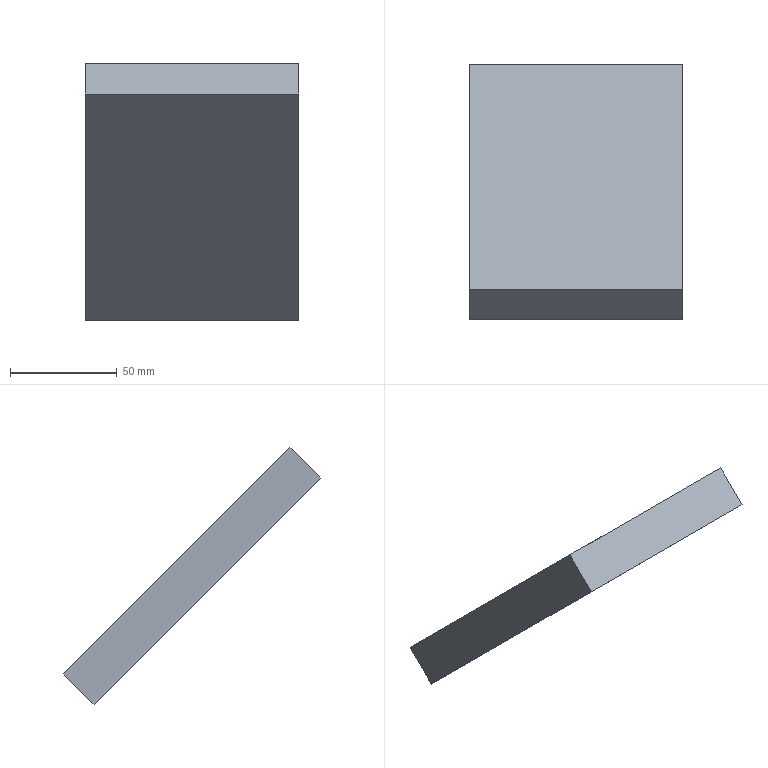Part | NX | features solid 2 | 1 solid | 6 faces | box 100 x 120.208 x 120.208 mm | volume 300000 mm3 | plane 6
STEP:
#1=CARTESIAN_POINT('',(730.,940.563,-169.939));
#2=VERTEX_POINT('',#1);
#3=CARTESIAN_POINT('',(730.,954.706,-155.797));
#4=VERTEX_POINT('',#3);
#5=CARTESIAN_POINT('',(730.,940.563,-169.939));
#6=DIRECTION('',(0.,0.7071,0.7071));
#7=VECTOR('',#6,1000.);
#8=LINE('',#5,#7);
#9=EDGE_CURVE('',#2,#4,#8,.T.);
#10=ORIENTED_EDGE('',*,*,#9,.T.);
#11=CARTESIAN_POINT('',(630.,954.706,-155.797));
#12=VERTEX_POINT('',#11);
#13=CARTESIAN_POINT('',(630.,954.706,-155.797));
#14=DIRECTION('',(1.,0.,0.));
#15=VECTOR('',#14,1000.);
#16=LINE('',#13,#15);
#17=EDGE_CURVE('',#12,#4,#16,.T.);
#18=ORIENTED_EDGE('',*,*,#17,.F.);
#19=CARTESIAN_POINT('',(630.,940.563,-169.939));
#20=VERTEX_POINT('',#19);
#21=CARTESIAN_POINT('',(630.,940.563,-169.939));
#22=DIRECTION('',(0.,0.7071,0.7071));
#23=VECTOR('',#22,1000.);
#24=LINE('',#21,#23);
#25=EDGE_CURVE('',#20,#12,#24,.T.);
#26=ORIENTED_EDGE('',*,*,#25,.F.);
#27=CARTESIAN_POINT('',(630.,940.563,-169.939));
#28=DIRECTION('',(1.,0.,0.));
#29=VECTOR('',#28,1000.);
#30=LINE('',#27,#29);
#31=EDGE_CURVE('',#20,#2,#30,.T.);
#32=ORIENTED_EDGE('',*,*,#31,.T.);
#33=EDGE_LOOP('',(#10,#18,#26,#32));
#34=FACE_BOUND('',#33,.T.);
#35=CARTESIAN_POINT('',(630.,940.563,-169.939));
#36=DIRECTION('',(0.,-0.7071,0.7071));
#37=DIRECTION('',(0.,-0.7071,-0.7071));
#38=AXIS2_PLACEMENT_3D('',#35,#36,#37);
#39=PLANE('',#38);
#40=ADVANCED_FACE('',(#34),#39,.T.);
#41=CARTESIAN_POINT('',(730.,1060.772,-261.863));
#42=VERTEX_POINT('',#41);
#43=CARTESIAN_POINT('',(730.,954.706,-155.797));
#44=DIRECTION('',(0.,0.7071,-0.7071));
#45=VECTOR('',#44,1000.);
#46=LINE('',#43,#45);
#47=EDGE_CURVE('',#4,#42,#46,.T.);
#48=ORIENTED_EDGE('',*,*,#47,.T.);
#49=CARTESIAN_POINT('',(630.,1060.772,-261.863));
#50=VERTEX_POINT('',#49);
#51=CARTESIAN_POINT('',(630.,1060.772,-261.863));
#52=DIRECTION('',(1.,0.,0.));
#53=VECTOR('',#52,1000.);
#54=LINE('',#51,#53);
#55=EDGE_CURVE('',#50,#42,#54,.T.);
#56=ORIENTED_EDGE('',*,*,#55,.F.);
#57=CARTESIAN_POINT('',(630.,954.706,-155.797));
#58=DIRECTION('',(0.,0.7071,-0.7071));
#59=VECTOR('',#58,1000.);
#60=LINE('',#57,#59);
#61=EDGE_CURVE('',#12,#50,#60,.T.);
#62=ORIENTED_EDGE('',*,*,#61,.F.);
#63=ORIENTED_EDGE('',*,*,#17,.T.);
#64=EDGE_LOOP('',(#48,#56,#62,#63));
#65=FACE_BOUND('',#64,.T.);
#66=CARTESIAN_POINT('',(630.,954.706,-155.797));
#67=DIRECTION('',(0.,0.7071,0.7071));
#68=DIRECTION('',(0.,-0.7071,0.7071));
#69=AXIS2_PLACEMENT_3D('',#66,#67,#68);
#70=PLANE('',#69);
#71=ADVANCED_FACE('',(#65),#70,.T.);
#72=CARTESIAN_POINT('',(730.,1046.63,-276.005));
#73=VERTEX_POINT('',#72);
#74=CARTESIAN_POINT('',(730.,1046.63,-276.005));
#75=DIRECTION('',(0.,0.7071,0.7071));
#76=VECTOR('',#75,1000.);
#77=LINE('',#74,#76);
#78=EDGE_CURVE('',#73,#42,#77,.T.);
#79=ORIENTED_EDGE('',*,*,#78,.F.);
#80=CARTESIAN_POINT('',(630.,1046.63,-276.005));
#81=VERTEX_POINT('',#80);
#82=CARTESIAN_POINT('',(630.,1046.63,-276.005));
#83=DIRECTION('',(1.,0.,0.));
#84=VECTOR('',#83,1000.);
#85=LINE('',#82,#84);
#86=EDGE_CURVE('',#81,#73,#85,.T.);
#87=ORIENTED_EDGE('',*,*,#86,.F.);
#88=CARTESIAN_POINT('',(630.,1046.63,-276.005));
#89=DIRECTION('',(0.,0.7071,0.7071));
#90=VECTOR('',#89,1000.);
#91=LINE('',#88,#90);
#92=EDGE_CURVE('',#81,#50,#91,.T.);
#93=ORIENTED_EDGE('',*,*,#92,.T.);
#94=ORIENTED_EDGE('',*,*,#55,.T.);
#95=EDGE_LOOP('',(#79,#87,#93,#94));
#96=FACE_BOUND('',#95,.T.);
#97=CARTESIAN_POINT('',(630.,1046.63,-276.005));
#98=DIRECTION('',(0.,-0.7071,0.7071));
#99=DIRECTION('',(0.,-0.7071,-0.7071));
#100=AXIS2_PLACEMENT_3D('',#97,#98,#99);
#101=PLANE('',#100);
#102=ADVANCED_FACE('',(#96),#101,.F.);
#103=CARTESIAN_POINT('',(730.,940.563,-169.939));
#104=DIRECTION('',(0.,0.7071,-0.7071));
#105=VECTOR('',#104,1000.);
#106=LINE('',#103,#105);
#107=EDGE_CURVE('',#2,#73,#106,.T.);
#108=ORIENTED_EDGE('',*,*,#107,.F.);
#109=ORIENTED_EDGE('',*,*,#31,.F.);
#110=CARTESIAN_POINT('',(630.,940.563,-169.939));
#111=DIRECTION('',(0.,0.7071,-0.7071));
#112=VECTOR('',#111,1000.);
#113=LINE('',#110,#112);
#114=EDGE_CURVE('',#20,#81,#113,.T.);
#115=ORIENTED_EDGE('',*,*,#114,.T.);
#116=ORIENTED_EDGE('',*,*,#86,.T.);
#117=EDGE_LOOP('',(#108,#109,#115,#116));
#118=FACE_BOUND('',#117,.T.);
#119=CARTESIAN_POINT('',(630.,940.563,-169.939));
#120=DIRECTION('',(0.,0.7071,0.7071));
#121=DIRECTION('',(0.,-0.7071,0.7071));
#122=AXIS2_PLACEMENT_3D('',#119,#120,#121);
#123=PLANE('',#122);
#124=ADVANCED_FACE('',(#118),#123,.F.);
#125=ORIENTED_EDGE('',*,*,#25,.T.);
#126=ORIENTED_EDGE('',*,*,#61,.T.);
#127=ORIENTED_EDGE('',*,*,#92,.F.);
#128=ORIENTED_EDGE('',*,*,#114,.F.);
#129=EDGE_LOOP('',(#125,#126,#127,#128));
#130=FACE_BOUND('',#129,.T.);
#131=CARTESIAN_POINT('',(630.,940.563,-169.939));
#132=DIRECTION('',(1.,0.,0.));
#133=DIRECTION('',(0.,0.,1.));
#134=AXIS2_PLACEMENT_3D('',#131,#132,#133);
#135=PLANE('',#134);
#136=ADVANCED_FACE('',(#130),#135,.F.);
#137=ORIENTED_EDGE('',*,*,#9,.F.);
#138=ORIENTED_EDGE('',*,*,#107,.T.);
#139=ORIENTED_EDGE('',*,*,#78,.T.);
#140=ORIENTED_EDGE('',*,*,#47,.F.);
#141=EDGE_LOOP('',(#137,#138,#139,#140));
#142=FACE_BOUND('',#141,.T.);
#143=CARTESIAN_POINT('',(730.,940.563,-169.939));
#144=DIRECTION('',(1.,0.,0.));
#145=DIRECTION('',(0.,0.,1.));
#146=AXIS2_PLACEMENT_3D('',#143,#144,#145);
#147=PLANE('',#146);
#148=ADVANCED_FACE('',(#142),#147,.T.);
#149=CLOSED_SHELL('',(#40,#71,#102,#124,#136,#148));
#150=MANIFOLD_SOLID_BREP('',#149);
#151=(LENGTH_UNIT()NAMED_UNIT(*)SI_UNIT(.MILLI.,.METRE.));
#152=UNCERTAINTY_MEASURE_WITH_UNIT(LENGTH_MEASURE(0.00001),#151,'','');
#153=(NAMED_UNIT(*)PLANE_ANGLE_UNIT()SI_UNIT($,.RADIAN.));
#154=(NAMED_UNIT(*)SI_UNIT($,.STERADIAN.)SOLID_ANGLE_UNIT());
#155=(GEOMETRIC_REPRESENTATION_CONTEXT(3)GLOBAL_UNCERTAINTY_ASSIGNED_CONTEXT((#152))GLOBAL_UNIT_ASSIGNED_CONTEXT((#151,#153,#154))REPRESENTATION_CONTEXT('',''));
#156=ADVANCED_BREP_SHAPE_REPRESENTATION('',(#150),#155);